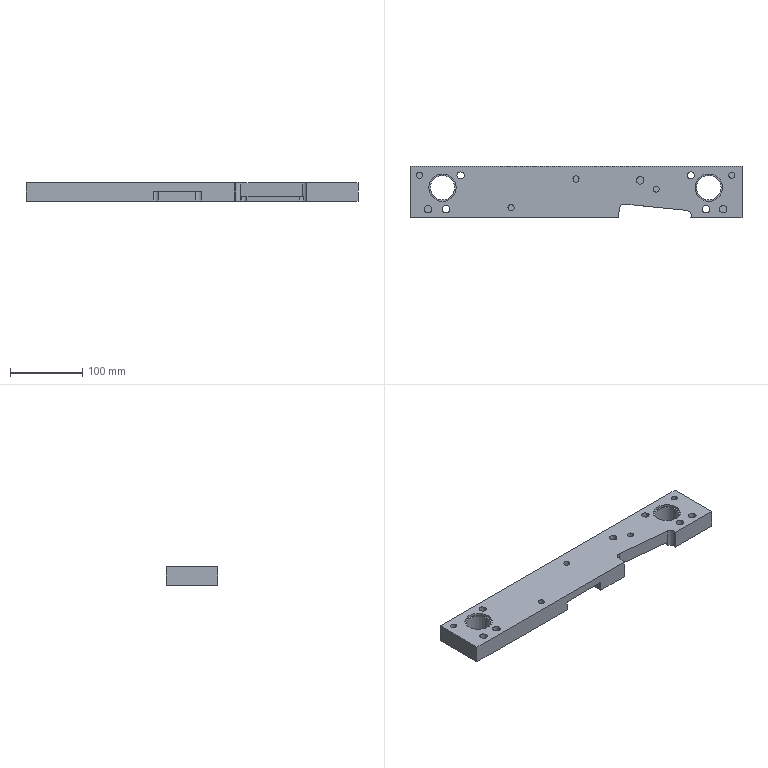Part | NX | features LIN_SOLID_COLOR 2 | 1 solid | 54 faces | box 460 x 72 x 25 mm | volume 694887 mm3 | plane 30 | cylinder 24 | commonest cylinder face diameters 8.5 x5 10.3 x5 10 x4 10.001 x2 10.31 x2 14 x2
STEP:
#1=CARTESIAN_POINT('',(698.25,138.,7.));
#2=VERTEX_POINT('',#1);
#3=CARTESIAN_POINT('',(694.,138.,7.));
#4=DIRECTION('',(0.,0.,1.));
#5=DIRECTION('',(1.,0.,0.));
#6=AXIS2_PLACEMENT_3D('',#3,#4,#5);
#7=CIRCLE('',#6,4.25);
#8=EDGE_CURVE('',#2,#2,#7,.F.);
#9=ORIENTED_EDGE('',*,*,#8,.T.);
#10=EDGE_LOOP('',(#9));
#11=FACE_BOUND('',#10,.T.);
#12=CARTESIAN_POINT('',(698.25,138.,25.));
#13=VERTEX_POINT('',#12);
#14=CARTESIAN_POINT('',(694.,138.,25.));
#15=DIRECTION('',(0.,0.,1.));
#16=DIRECTION('',(1.,0.,0.));
#17=AXIS2_PLACEMENT_3D('',#14,#15,#16);
#18=CIRCLE('',#17,4.25);
#19=EDGE_CURVE('',#13,#13,#18,.T.);
#20=ORIENTED_EDGE('',*,*,#19,.T.);
#21=EDGE_LOOP('',(#20));
#22=FACE_BOUND('',#21,.T.);
#23=CARTESIAN_POINT('',(694.,138.,25.1));
#24=DIRECTION('',(0.,0.,-1.));
#25=DIRECTION('',(1.,0.,0.));
#26=AXIS2_PLACEMENT_3D('',#23,#24,#25);
#27=CYLINDRICAL_SURFACE('',#26,4.25);
#28=ADVANCED_FACE('',(#11,#22),#27,.F.);
#29=CARTESIAN_POINT('',(747.152,157.,0.));
#30=VERTEX_POINT('',#29);
#31=CARTESIAN_POINT('',(741.997,157.,0.));
#32=DIRECTION('',(0.,0.,1.));
#33=DIRECTION('',(1.,0.,0.));
#34=AXIS2_PLACEMENT_3D('',#31,#32,#33);
#35=CIRCLE('',#34,5.155);
#36=EDGE_CURVE('',#30,#30,#35,.T.);
#37=ORIENTED_EDGE('',*,*,#36,.T.);
#38=EDGE_LOOP('',(#37));
#39=FACE_BOUND('',#38,.T.);
#40=CARTESIAN_POINT('',(428.158,157.,0.));
#41=VERTEX_POINT('',#40);
#42=CARTESIAN_POINT('',(423.003,157.,0.));
#43=DIRECTION('',(0.,0.,1.));
#44=DIRECTION('',(1.,0.,0.));
#45=AXIS2_PLACEMENT_3D('',#42,#43,#44);
#46=CIRCLE('',#45,5.155);
#47=EDGE_CURVE('',#41,#41,#46,.T.);
#48=ORIENTED_EDGE('',*,*,#47,.T.);
#49=EDGE_LOOP('',(#48));
#50=FACE_BOUND('',#49,.T.);
#51=CARTESIAN_POINT('',(757.85,110.,0.));
#52=VERTEX_POINT('',#51);
#53=CARTESIAN_POINT('',(763.,110.,0.));
#54=DIRECTION('',(0.,0.,-1.));
#55=DIRECTION('',(-1.,0.,0.));
#56=AXIS2_PLACEMENT_3D('',#53,#54,#55);
#57=CIRCLE('',#56,5.15);
#58=EDGE_CURVE('',#52,#52,#57,.T.);
#59=ORIENTED_EDGE('',*,*,#58,.F.);
#60=EDGE_LOOP('',(#59));
#61=FACE_BOUND('',#60,.T.);
#62=CARTESIAN_POINT('',(397.85,110.,0.));
#63=VERTEX_POINT('',#62);
#64=CARTESIAN_POINT('',(403.,110.,0.));
#65=DIRECTION('',(0.,0.,-1.));
#66=DIRECTION('',(-1.,0.,0.));
#67=AXIS2_PLACEMENT_3D('',#64,#65,#66);
#68=CIRCLE('',#67,5.15);
#69=EDGE_CURVE('',#63,#63,#68,.T.);
#70=ORIENTED_EDGE('',*,*,#69,.F.);
#71=EDGE_LOOP('',(#70));
#72=FACE_BOUND('',#71,.T.);
#73=CARTESIAN_POINT('',(381.,140.,0.));
#74=VERTEX_POINT('',#73);
#75=CARTESIAN_POINT('',(398.,140.,0.));
#76=DIRECTION('',(0.,0.,-1.));
#77=DIRECTION('',(-1.,0.,0.));
#78=AXIS2_PLACEMENT_3D('',#75,#76,#77);
#79=CIRCLE('',#78,17.);
#80=EDGE_CURVE('',#74,#74,#79,.T.);
#81=ORIENTED_EDGE('',*,*,#80,.F.);
#82=EDGE_LOOP('',(#81));
#83=FACE_BOUND('',#82,.T.);
#84=CARTESIAN_POINT('',(750.,140.,0.));
#85=VERTEX_POINT('',#84);
#86=CARTESIAN_POINT('',(767.,140.,0.));
#87=DIRECTION('',(0.,0.,-1.));
#88=DIRECTION('',(-1.,0.,0.));
#89=AXIS2_PLACEMENT_3D('',#86,#87,#88);
#90=CIRCLE('',#89,17.);
#91=EDGE_CURVE('',#85,#85,#90,.T.);
#92=ORIENTED_EDGE('',*,*,#91,.F.);
#93=EDGE_LOOP('',(#92));
#94=FACE_BOUND('',#93,.T.);
#95=CARTESIAN_POINT('',(650.988,129.15,0.));
#96=VERTEX_POINT('',#95);
#97=CARTESIAN_POINT('',(658.697,135.448,0.));
#98=VERTEX_POINT('',#97);
#99=CARTESIAN_POINT('',(654.541,132.668,0.));
#100=DIRECTION('',(0.,0.,-1.));
#101=DIRECTION('',(-1.,0.,0.));
#102=AXIS2_PLACEMENT_3D('',#99,#100,#101);
#103=CIRCLE('',#102,5.);
#104=EDGE_CURVE('',#96,#98,#103,.T.);
#105=ORIENTED_EDGE('',*,*,#104,.F.);
#106=CARTESIAN_POINT('',(649.783,117.177,0.));
#107=VERTEX_POINT('',#106);
#108=CARTESIAN_POINT('',(639.027,10.37,0.));
#109=DIRECTION('',(0.1002,0.995,0.));
#110=VECTOR('',#109,1000.);
#111=LINE('',#108,#110);
#112=EDGE_CURVE('',#107,#96,#111,.T.);
#113=ORIENTED_EDGE('',*,*,#112,.F.);
#114=CARTESIAN_POINT('',(643.119,110.885,0.));
#115=VERTEX_POINT('',#114);
#116=CARTESIAN_POINT('',(650.083,110.184,0.));
#117=DIRECTION('',(0.,0.,-1.));
#118=DIRECTION('',(-1.,0.,0.));
#119=AXIS2_PLACEMENT_3D('',#116,#117,#118);
#120=CIRCLE('',#119,7.);
#121=EDGE_CURVE('',#115,#107,#120,.T.);
#122=ORIENTED_EDGE('',*,*,#121,.F.);
#123=CARTESIAN_POINT('',(641.821,98.,0.));
#124=VERTEX_POINT('',#123);
#125=CARTESIAN_POINT('',(633.057,10.971,0.));
#126=DIRECTION('',(0.1002,0.995,0.));
#127=VECTOR('',#126,1000.);
#128=LINE('',#125,#127);
#129=EDGE_CURVE('',#124,#115,#128,.T.);
#130=ORIENTED_EDGE('',*,*,#129,.F.);
#131=CARTESIAN_POINT('',(595.5,98.,0.));
#132=VERTEX_POINT('',#131);
#133=CARTESIAN_POINT('',(742.,98.,0.));
#134=DIRECTION('',(-1.,0.,0.));
#135=VECTOR('',#134,1000.);
#136=LINE('',#133,#135);
#137=EDGE_CURVE('',#124,#132,#136,.T.);
#138=ORIENTED_EDGE('',*,*,#137,.T.);
#139=CARTESIAN_POINT('',(595.5,111.161,0.));
#140=VERTEX_POINT('',#139);
#141=CARTESIAN_POINT('',(595.5,0.,0.));
#142=DIRECTION('',(0.,1.,0.));
#143=VECTOR('',#142,1000.);
#144=LINE('',#141,#143);
#145=EDGE_CURVE('',#132,#140,#144,.T.);
#146=ORIENTED_EDGE('',*,*,#145,.T.);
#147=CARTESIAN_POINT('',(588.461,118.2,0.));
#148=VERTEX_POINT('',#147);
#149=CARTESIAN_POINT('',(592.318,115.018,0.));
#150=DIRECTION('',(0.,0.,-1.));
#151=DIRECTION('',(-1.,0.,0.));
#152=AXIS2_PLACEMENT_3D('',#149,#150,#151);
#153=CIRCLE('',#152,5.);
#154=EDGE_CURVE('',#140,#148,#153,.F.);
#155=ORIENTED_EDGE('',*,*,#154,.T.);
#156=CARTESIAN_POINT('',(536.539,118.2,0.));
#157=VERTEX_POINT('',#156);
#158=CARTESIAN_POINT('',(742.,118.2,0.));
#159=DIRECTION('',(-1.,0.,0.));
#160=VECTOR('',#159,1000.);
#161=LINE('',#158,#160);
#162=EDGE_CURVE('',#148,#157,#161,.T.);
#163=ORIENTED_EDGE('',*,*,#162,.T.);
#164=CARTESIAN_POINT('',(529.5,111.161,0.));
#165=VERTEX_POINT('',#164);
#166=CARTESIAN_POINT('',(532.682,115.018,0.));
#167=DIRECTION('',(0.,0.,-1.));
#168=DIRECTION('',(-1.,0.,0.));
#169=AXIS2_PLACEMENT_3D('',#166,#167,#168);
#170=CIRCLE('',#169,5.);
#171=EDGE_CURVE('',#157,#165,#170,.F.);
#172=ORIENTED_EDGE('',*,*,#171,.T.);
#173=CARTESIAN_POINT('',(529.5,98.,0.));
#174=VERTEX_POINT('',#173);
#175=CARTESIAN_POINT('',(529.5,0.,0.));
#176=DIRECTION('',(0.,-1.,0.));
#177=VECTOR('',#176,1000.);
#178=LINE('',#175,#177);
#179=EDGE_CURVE('',#165,#174,#178,.T.);
#180=ORIENTED_EDGE('',*,*,#179,.T.);
#181=CARTESIAN_POINT('',(353.,98.,0.));
#182=VERTEX_POINT('',#181);
#183=CARTESIAN_POINT('',(742.,98.,0.));
#184=DIRECTION('',(-1.,0.,0.));
#185=VECTOR('',#184,1000.);
#186=LINE('',#183,#185);
#187=EDGE_CURVE('',#174,#182,#186,.T.);
#188=ORIENTED_EDGE('',*,*,#187,.T.);
#189=CARTESIAN_POINT('',(353.,170.,0.));
#190=VERTEX_POINT('',#189);
#191=CARTESIAN_POINT('',(353.,0.,0.));
#192=DIRECTION('',(0.,-1.,0.));
#193=VECTOR('',#192,1000.);
#194=LINE('',#191,#193);
#195=EDGE_CURVE('',#190,#182,#194,.T.);
#196=ORIENTED_EDGE('',*,*,#195,.F.);
#197=CARTESIAN_POINT('',(813.,170.,0.));
#198=VERTEX_POINT('',#197);
#199=CARTESIAN_POINT('',(788.,170.,0.));
#200=DIRECTION('',(-1.,0.,0.));
#201=VECTOR('',#200,1000.);
#202=LINE('',#199,#201);
#203=EDGE_CURVE('',#198,#190,#202,.T.);
#204=ORIENTED_EDGE('',*,*,#203,.F.);
#205=CARTESIAN_POINT('',(813.,98.,0.));
#206=VERTEX_POINT('',#205);
#207=CARTESIAN_POINT('',(813.,0.,0.));
#208=DIRECTION('',(0.,-1.,0.));
#209=VECTOR('',#208,1000.);
#210=LINE('',#207,#209);
#211=EDGE_CURVE('',#198,#206,#210,.T.);
#212=ORIENTED_EDGE('',*,*,#211,.T.);
#213=CARTESIAN_POINT('',(742.327,98.,0.));
#214=VERTEX_POINT('',#213);
#215=CARTESIAN_POINT('',(742.,98.,0.));
#216=DIRECTION('',(-1.,0.,0.));
#217=VECTOR('',#216,1000.);
#218=LINE('',#215,#217);
#219=EDGE_CURVE('',#206,#214,#218,.T.);
#220=ORIENTED_EDGE('',*,*,#219,.T.);
#221=CARTESIAN_POINT('',(742.615,100.865,0.));
#222=VERTEX_POINT('',#221);
#223=CARTESIAN_POINT('',(732.553,0.9513,0.));
#224=DIRECTION('',(-0.1002,-0.995,0.));
#225=VECTOR('',#224,1000.);
#226=LINE('',#223,#225);
#227=EDGE_CURVE('',#222,#214,#226,.T.);
#228=ORIENTED_EDGE('',*,*,#227,.F.);
#229=CARTESIAN_POINT('',(737.34,108.36,0.));
#230=VERTEX_POINT('',#229);
#231=CARTESIAN_POINT('',(735.651,101.567,0.));
#232=DIRECTION('',(0.,0.,-1.));
#233=DIRECTION('',(-1.,0.,0.));
#234=AXIS2_PLACEMENT_3D('',#231,#232,#233);
#235=CIRCLE('',#234,7.);
#236=EDGE_CURVE('',#230,#222,#235,.T.);
#237=ORIENTED_EDGE('',*,*,#236,.F.);
#238=CARTESIAN_POINT('',(738.545,120.332,0.));
#239=VERTEX_POINT('',#238);
#240=CARTESIAN_POINT('',(726.584,1.552,0.));
#241=DIRECTION('',(-0.1002,-0.995,0.));
#242=VECTOR('',#241,1000.);
#243=LINE('',#240,#242);
#244=EDGE_CURVE('',#239,#230,#243,.T.);
#245=ORIENTED_EDGE('',*,*,#244,.F.);
#246=CARTESIAN_POINT('',(732.247,128.041,0.));
#247=VERTEX_POINT('',#246);
#248=CARTESIAN_POINT('',(735.766,124.489,0.));
#249=DIRECTION('',(0.,0.,-1.));
#250=DIRECTION('',(-1.,0.,0.));
#251=AXIS2_PLACEMENT_3D('',#248,#249,#250);
#252=CIRCLE('',#251,5.);
#253=EDGE_CURVE('',#247,#239,#252,.T.);
#254=ORIENTED_EDGE('',*,*,#253,.F.);
#255=CARTESIAN_POINT('',(754.667,125.783,0.));
#256=DIRECTION('',(0.995,-0.1002,0.));
#257=VECTOR('',#256,1000.);
#258=LINE('',#255,#257);
#259=EDGE_CURVE('',#98,#247,#258,.T.);
#260=ORIENTED_EDGE('',*,*,#259,.F.);
#261=EDGE_LOOP('',(#105,#113,#122,#130,#138,#146,#155,#163,#172,#180,#188,#196,#204,#212,#220,#228,#237,#245,#254,#260));
#262=FACE_BOUND('',#261,.T.);
#263=CARTESIAN_POINT('',(742.,0.,0.));
#264=DIRECTION('',(0.,0.,-1.));
#265=DIRECTION('',(-1.,0.,0.));
#266=AXIS2_PLACEMENT_3D('',#263,#264,#265);
#267=PLANE('',#266);
#268=ADVANCED_FACE('',(#39,#50,#61,#72,#83,#94,#262),#267,.T.);
#269=CARTESIAN_POINT('',(587.25,152.,1.));
#270=VERTEX_POINT('',#269);
#271=CARTESIAN_POINT('',(583.,152.,1.));
#272=DIRECTION('',(0.,0.,1.));
#273=DIRECTION('',(1.,0.,0.));
#274=AXIS2_PLACEMENT_3D('',#271,#272,#273);
#275=CIRCLE('',#274,4.25);
#276=EDGE_CURVE('',#270,#270,#275,.F.);
#277=ORIENTED_EDGE('',*,*,#276,.T.);
#278=EDGE_LOOP('',(#277));
#279=FACE_BOUND('',#278,.T.);
#280=CARTESIAN_POINT('',(587.25,152.,25.));
#281=VERTEX_POINT('',#280);
#282=CARTESIAN_POINT('',(583.,152.,25.));
#283=DIRECTION('',(0.,0.,1.));
#284=DIRECTION('',(1.,0.,0.));
#285=AXIS2_PLACEMENT_3D('',#282,#283,#284);
#286=CIRCLE('',#285,4.25);
#287=EDGE_CURVE('',#281,#281,#286,.T.);
#288=ORIENTED_EDGE('',*,*,#287,.T.);
#289=EDGE_LOOP('',(#288));
#290=FACE_BOUND('',#289,.T.);
#291=CARTESIAN_POINT('',(583.,152.,25.1));
#292=DIRECTION('',(0.,0.,-1.));
#293=DIRECTION('',(1.,0.,0.));
#294=AXIS2_PLACEMENT_3D('',#291,#292,#293);
#295=CYLINDRICAL_SURFACE('',#294,4.25);
#296=ADVANCED_FACE('',(#279,#290),#295,.F.);
#297=CARTESIAN_POINT('',(595.5,111.161,13.5));
#298=VERTEX_POINT('',#297);
#299=CARTESIAN_POINT('',(588.461,118.2,13.5));
#300=VERTEX_POINT('',#299);
#301=CARTESIAN_POINT('',(592.318,115.018,13.5));
#302=DIRECTION('',(0.,0.,1.));
#303=DIRECTION('',(1.,0.,0.));
#304=AXIS2_PLACEMENT_3D('',#301,#302,#303);
#305=CIRCLE('',#304,5.);
#306=EDGE_CURVE('',#298,#300,#305,.T.);
#307=ORIENTED_EDGE('',*,*,#306,.F.);
#308=CARTESIAN_POINT('',(595.5,98.,13.5));
#309=VERTEX_POINT('',#308);
#310=CARTESIAN_POINT('',(595.5,90.2,13.5));
#311=DIRECTION('',(0.,1.,0.));
#312=VECTOR('',#311,1000.);
#313=LINE('',#310,#312);
#314=EDGE_CURVE('',#309,#298,#313,.T.);
#315=ORIENTED_EDGE('',*,*,#314,.F.);
#316=CARTESIAN_POINT('',(529.5,98.,13.5));
#317=VERTEX_POINT('',#316);
#318=CARTESIAN_POINT('',(915.758,98.,13.5));
#319=DIRECTION('',(-1.,0.,0.));
#320=VECTOR('',#319,1000.);
#321=LINE('',#318,#320);
#322=EDGE_CURVE('',#309,#317,#321,.T.);
#323=ORIENTED_EDGE('',*,*,#322,.T.);
#324=CARTESIAN_POINT('',(529.5,111.161,13.5));
#325=VERTEX_POINT('',#324);
#326=CARTESIAN_POINT('',(529.5,110.2,13.5));
#327=DIRECTION('',(0.,-1.,0.));
#328=VECTOR('',#327,1000.);
#329=LINE('',#326,#328);
#330=EDGE_CURVE('',#325,#317,#329,.T.);
#331=ORIENTED_EDGE('',*,*,#330,.F.);
#332=CARTESIAN_POINT('',(536.539,118.2,13.5));
#333=VERTEX_POINT('',#332);
#334=CARTESIAN_POINT('',(532.682,115.018,13.5));
#335=DIRECTION('',(0.,0.,1.));
#336=DIRECTION('',(1.,0.,0.));
#337=AXIS2_PLACEMENT_3D('',#334,#335,#336);
#338=CIRCLE('',#337,5.);
#339=EDGE_CURVE('',#333,#325,#338,.T.);
#340=ORIENTED_EDGE('',*,*,#339,.F.);
#341=CARTESIAN_POINT('',(572.,118.2,13.5));
#342=DIRECTION('',(-1.,0.,0.));
#343=VECTOR('',#342,1000.);
#344=LINE('',#341,#343);
#345=EDGE_CURVE('',#300,#333,#344,.T.);
#346=ORIENTED_EDGE('',*,*,#345,.F.);
#347=EDGE_LOOP('',(#307,#315,#323,#331,#340,#346));
#348=FACE_BOUND('',#347,.T.);
#349=CARTESIAN_POINT('',(552.555,107.951,13.5));
#350=DIRECTION('',(0.,0.,1.));
#351=DIRECTION('',(1.,0.,0.));
#352=AXIS2_PLACEMENT_3D('',#349,#350,#351);
#353=PLANE('',#352);
#354=ADVANCED_FACE('',(#348),#353,.F.);
#355=CARTESIAN_POINT('',(415.,140.,21.7));
#356=VERTEX_POINT('',#355);
#357=CARTESIAN_POINT('',(398.,140.,21.7));
#358=DIRECTION('',(0.,0.,1.));
#359=DIRECTION('',(1.,0.,0.));
#360=AXIS2_PLACEMENT_3D('',#357,#358,#359);
#361=CIRCLE('',#360,17.);
#362=EDGE_CURVE('',#356,#356,#361,.F.);
#363=ORIENTED_EDGE('',*,*,#362,.T.);
#364=EDGE_LOOP('',(#363));
#365=FACE_BOUND('',#364,.T.);
#366=CARTESIAN_POINT('',(417.,140.,21.7));
#367=VERTEX_POINT('',#366);
#368=CARTESIAN_POINT('',(398.,140.,21.7));
#369=DIRECTION('',(0.,0.,1.));
#370=DIRECTION('',(1.,0.,0.));
#371=AXIS2_PLACEMENT_3D('',#368,#369,#370);
#372=CIRCLE('',#371,19.);
#373=EDGE_CURVE('',#367,#367,#372,.F.);
#374=ORIENTED_EDGE('',*,*,#373,.F.);
#375=EDGE_LOOP('',(#374));
#376=FACE_BOUND('',#375,.T.);
#377=CARTESIAN_POINT('',(398.,140.,21.7));
#378=DIRECTION('',(0.,0.,1.));
#379=DIRECTION('',(1.,0.,0.));
#380=AXIS2_PLACEMENT_3D('',#377,#378,#379);
#381=PLANE('',#380);
#382=ADVANCED_FACE('',(#365,#376),#381,.T.);
#383=CARTESIAN_POINT('',(784.,140.,21.7));
#384=VERTEX_POINT('',#383);
#385=CARTESIAN_POINT('',(767.,140.,21.7));
#386=DIRECTION('',(0.,0.,1.));
#387=DIRECTION('',(1.,0.,0.));
#388=AXIS2_PLACEMENT_3D('',#385,#386,#387);
#389=CIRCLE('',#388,17.);
#390=EDGE_CURVE('',#384,#384,#389,.F.);
#391=ORIENTED_EDGE('',*,*,#390,.T.);
#392=EDGE_LOOP('',(#391));
#393=FACE_BOUND('',#392,.T.);
#394=CARTESIAN_POINT('',(786.,140.,21.7));
#395=VERTEX_POINT('',#394);
#396=CARTESIAN_POINT('',(767.,140.,21.7));
#397=DIRECTION('',(0.,0.,1.));
#398=DIRECTION('',(1.,0.,0.));
#399=AXIS2_PLACEMENT_3D('',#396,#397,#398);
#400=CIRCLE('',#399,19.);
#401=EDGE_CURVE('',#395,#395,#400,.F.);
#402=ORIENTED_EDGE('',*,*,#401,.F.);
#403=EDGE_LOOP('',(#402));
#404=FACE_BOUND('',#403,.T.);
#405=CARTESIAN_POINT('',(767.,140.,21.7));
#406=DIRECTION('',(0.,0.,1.));
#407=DIRECTION('',(1.,0.,0.));
#408=AXIS2_PLACEMENT_3D('',#405,#406,#407);
#409=PLANE('',#408);
#410=ADVANCED_FACE('',(#393,#404),#409,.T.);
#411=CARTESIAN_POINT('',(786.,140.,25.));
#412=VERTEX_POINT('',#411);
#413=CARTESIAN_POINT('',(767.,140.,25.));
#414=DIRECTION('',(0.,0.,1.));
#415=DIRECTION('',(1.,0.,0.));
#416=AXIS2_PLACEMENT_3D('',#413,#414,#415);
#417=CIRCLE('',#416,19.);
#418=EDGE_CURVE('',#412,#412,#417,.T.);
#419=ORIENTED_EDGE('',*,*,#418,.T.);
#420=EDGE_LOOP('',(#419));
#421=FACE_BOUND('',#420,.T.);
#422=ORIENTED_EDGE('',*,*,#401,.T.);
#423=EDGE_LOOP('',(#422));
#424=FACE_BOUND('',#423,.T.);
#425=CARTESIAN_POINT('',(767.,140.,21.5));
#426=DIRECTION('',(0.,0.,1.));
#427=DIRECTION('',(1.,0.,0.));
#428=AXIS2_PLACEMENT_3D('',#425,#426,#427);
#429=CYLINDRICAL_SURFACE('',#428,19.);
#430=ADVANCED_FACE('',(#421,#424),#429,.F.);
#431=CARTESIAN_POINT('',(417.,140.,25.));
#432=VERTEX_POINT('',#431);
#433=CARTESIAN_POINT('',(398.,140.,25.));
#434=DIRECTION('',(0.,0.,1.));
#435=DIRECTION('',(1.,0.,0.));
#436=AXIS2_PLACEMENT_3D('',#433,#434,#435);
#437=CIRCLE('',#436,19.);
#438=EDGE_CURVE('',#432,#432,#437,.T.);
#439=ORIENTED_EDGE('',*,*,#438,.T.);
#440=EDGE_LOOP('',(#439));
#441=FACE_BOUND('',#440,.T.);
#442=ORIENTED_EDGE('',*,*,#373,.T.);
#443=EDGE_LOOP('',(#442));
#444=FACE_BOUND('',#443,.T.);
#445=CARTESIAN_POINT('',(398.,140.,21.5));
#446=DIRECTION('',(0.,0.,1.));
#447=DIRECTION('',(1.,0.,0.));
#448=AXIS2_PLACEMENT_3D('',#445,#446,#447);
#449=CYLINDRICAL_SURFACE('',#448,19.);
#450=ADVANCED_FACE('',(#441,#444),#449,.F.);
#451=CARTESIAN_POINT('',(588.461,118.2,-46.5));
#452=DIRECTION('',(0.,0.,1.));
#453=VECTOR('',#452,1000.);
#454=LINE('',#451,#453);
#455=EDGE_CURVE('',#148,#300,#454,.T.);
#456=ORIENTED_EDGE('',*,*,#455,.T.);
#457=ORIENTED_EDGE('',*,*,#345,.T.);
#458=CARTESIAN_POINT('',(536.539,118.2,-46.5));
#459=DIRECTION('',(0.,0.,1.));
#460=VECTOR('',#459,1000.);
#461=LINE('',#458,#460);
#462=EDGE_CURVE('',#157,#333,#461,.T.);
#463=ORIENTED_EDGE('',*,*,#462,.F.);
#464=ORIENTED_EDGE('',*,*,#162,.F.);
#465=EDGE_LOOP('',(#456,#457,#463,#464));
#466=FACE_BOUND('',#465,.T.);
#467=CARTESIAN_POINT('',(572.,118.2,-46.5));
#468=DIRECTION('',(0.,-1.,0.));
#469=DIRECTION('',(0.,0.,1.));
#470=AXIS2_PLACEMENT_3D('',#467,#468,#469);
#471=PLANE('',#470);
#472=ADVANCED_FACE('',(#466),#471,.T.);
#473=CARTESIAN_POINT('',(595.5,111.161,-46.5));
#474=DIRECTION('',(0.,0.,1.));
#475=VECTOR('',#474,1000.);
#476=LINE('',#473,#475);
#477=EDGE_CURVE('',#140,#298,#476,.T.);
#478=ORIENTED_EDGE('',*,*,#477,.T.);
#479=ORIENTED_EDGE('',*,*,#306,.T.);
#480=ORIENTED_EDGE('',*,*,#455,.F.);
#481=ORIENTED_EDGE('',*,*,#154,.F.);
#482=EDGE_LOOP('',(#478,#479,#480,#481));
#483=FACE_BOUND('',#482,.T.);
#484=CARTESIAN_POINT('',(592.318,115.018,-46.5));
#485=DIRECTION('',(0.,0.,1.));
#486=DIRECTION('',(1.,0.,0.));
#487=AXIS2_PLACEMENT_3D('',#484,#485,#486);
#488=CYLINDRICAL_SURFACE('',#487,5.);
#489=ADVANCED_FACE('',(#483),#488,.F.);
#490=CARTESIAN_POINT('',(595.5,98.,0.));
#491=DIRECTION('',(0.,0.,-1.));
#492=VECTOR('',#491,1000.);
#493=LINE('',#490,#492);
#494=EDGE_CURVE('',#309,#132,#493,.T.);
#495=ORIENTED_EDGE('',*,*,#494,.F.);
#496=ORIENTED_EDGE('',*,*,#314,.T.);
#497=ORIENTED_EDGE('',*,*,#477,.F.);
#498=ORIENTED_EDGE('',*,*,#145,.F.);
#499=EDGE_LOOP('',(#495,#496,#497,#498));
#500=FACE_BOUND('',#499,.T.);
#501=CARTESIAN_POINT('',(595.5,90.2,-46.5));
#502=DIRECTION('',(-1.,0.,0.));
#503=DIRECTION('',(0.,0.,1.));
#504=AXIS2_PLACEMENT_3D('',#501,#502,#503);
#505=PLANE('',#504);
#506=ADVANCED_FACE('',(#500),#505,.T.);
#507=CARTESIAN_POINT('',(643.119,110.885,25.));
#508=VERTEX_POINT('',#507);
#509=CARTESIAN_POINT('',(641.821,98.,25.));
#510=VERTEX_POINT('',#509);
#511=CARTESIAN_POINT('',(633.519,15.557,25.));
#512=DIRECTION('',(-0.1002,-0.995,0.));
#513=VECTOR('',#512,1000.);
#514=LINE('',#511,#513);
#515=EDGE_CURVE('',#508,#510,#514,.T.);
#516=ORIENTED_EDGE('',*,*,#515,.T.);
#517=CARTESIAN_POINT('',(641.821,98.,0.));
#518=DIRECTION('',(0.,0.,-1.));
#519=VECTOR('',#518,1000.);
#520=LINE('',#517,#519);
#521=EDGE_CURVE('',#510,#124,#520,.T.);
#522=ORIENTED_EDGE('',*,*,#521,.T.);
#523=ORIENTED_EDGE('',*,*,#129,.T.);
#524=CARTESIAN_POINT('',(643.119,110.885,-41.49));
#525=DIRECTION('',(0.,0.,1.));
#526=VECTOR('',#525,1000.);
#527=LINE('',#524,#526);
#528=EDGE_CURVE('',#115,#508,#527,.T.);
#529=ORIENTED_EDGE('',*,*,#528,.T.);
#530=EDGE_LOOP('',(#516,#522,#523,#529));
#531=FACE_BOUND('',#530,.T.);
#532=CARTESIAN_POINT('',(643.119,110.885,-41.49));
#533=DIRECTION('',(-0.995,0.1002,0.));
#534=DIRECTION('',(-0.1002,-0.995,0.));
#535=AXIS2_PLACEMENT_3D('',#532,#533,#534);
#536=PLANE('',#535);
#537=ADVANCED_FACE('',(#531),#536,.F.);
#538=CARTESIAN_POINT('',(649.783,117.177,6.));
#539=VERTEX_POINT('',#538);
#540=CARTESIAN_POINT('',(649.783,117.177,-41.49));
#541=DIRECTION('',(0.,0.,1.));
#542=VECTOR('',#541,1000.);
#543=LINE('',#540,#542);
#544=EDGE_CURVE('',#107,#539,#543,.T.);
#545=ORIENTED_EDGE('',*,*,#544,.T.);
#546=CARTESIAN_POINT('',(650.785,117.149,6.));
#547=VERTEX_POINT('',#546);
#548=CARTESIAN_POINT('',(650.083,110.184,6.));
#549=DIRECTION('',(0.,0.,1.));
#550=DIRECTION('',(1.,0.,0.));
#551=AXIS2_PLACEMENT_3D('',#548,#549,#550);
#552=CIRCLE('',#551,7.);
#553=EDGE_CURVE('',#539,#547,#552,.F.);
#554=ORIENTED_EDGE('',*,*,#553,.T.);
#555=CARTESIAN_POINT('',(650.785,117.149,25.));
#556=VERTEX_POINT('',#555);
#557=CARTESIAN_POINT('',(650.785,117.149,-41.49));
#558=DIRECTION('',(0.,0.,1.));
#559=VECTOR('',#558,1000.);
#560=LINE('',#557,#559);
#561=EDGE_CURVE('',#556,#547,#560,.F.);
#562=ORIENTED_EDGE('',*,*,#561,.F.);
#563=CARTESIAN_POINT('',(650.083,110.184,25.));
#564=DIRECTION('',(0.,0.,1.));
#565=DIRECTION('',(1.,0.,0.));
#566=AXIS2_PLACEMENT_3D('',#563,#564,#565);
#567=CIRCLE('',#566,7.);
#568=EDGE_CURVE('',#556,#508,#567,.T.);
#569=ORIENTED_EDGE('',*,*,#568,.T.);
#570=ORIENTED_EDGE('',*,*,#528,.F.);
#571=ORIENTED_EDGE('',*,*,#121,.T.);
#572=EDGE_LOOP('',(#545,#554,#562,#569,#570,#571));
#573=FACE_BOUND('',#572,.T.);
#574=CARTESIAN_POINT('',(650.083,110.184,-41.49));
#575=DIRECTION('',(0.,0.,1.));
#576=DIRECTION('',(1.,0.,0.));
#577=AXIS2_PLACEMENT_3D('',#574,#575,#576);
#578=CYLINDRICAL_SURFACE('',#577,7.);
#579=ADVANCED_FACE('',(#573),#578,.F.);
#580=CARTESIAN_POINT('',(736.352,108.532,6.));
#581=VERTEX_POINT('',#580);
#582=CARTESIAN_POINT('',(652.775,116.948,6.));
#583=DIRECTION('',(-0.995,0.1002,0.));
#584=VECTOR('',#583,1000.);
#585=LINE('',#582,#584);
#586=EDGE_CURVE('',#581,#547,#585,.T.);
#587=ORIENTED_EDGE('',*,*,#586,.F.);
#588=CARTESIAN_POINT('',(736.352,108.532,25.));
#589=VERTEX_POINT('',#588);
#590=CARTESIAN_POINT('',(736.352,108.532,-41.49));
#591=DIRECTION('',(0.,0.,1.));
#592=VECTOR('',#591,1000.);
#593=LINE('',#590,#592);
#594=EDGE_CURVE('',#581,#589,#593,.T.);
#595=ORIENTED_EDGE('',*,*,#594,.T.);
#596=CARTESIAN_POINT('',(798.301,102.293,25.));
#597=DIRECTION('',(0.995,-0.1002,0.));
#598=VECTOR('',#597,1000.);
#599=LINE('',#596,#598);
#600=EDGE_CURVE('',#556,#589,#599,.T.);
#601=ORIENTED_EDGE('',*,*,#600,.F.);
#602=ORIENTED_EDGE('',*,*,#561,.T.);
#603=EDGE_LOOP('',(#587,#595,#601,#602));
#604=FACE_BOUND('',#603,.T.);
#605=CARTESIAN_POINT('',(652.775,116.948,-41.49));
#606=DIRECTION('',(-0.1002,-0.995,0.));
#607=DIRECTION('',(0.995,-0.1002,0.));
#608=AXIS2_PLACEMENT_3D('',#605,#606,#607);
#609=PLANE('',#608);
#610=ADVANCED_FACE('',(#604),#609,.T.);
#611=ORIENTED_EDGE('',*,*,#594,.F.);
#612=CARTESIAN_POINT('',(737.34,108.36,6.));
#613=VERTEX_POINT('',#612);
#614=CARTESIAN_POINT('',(735.651,101.567,6.));
#615=DIRECTION('',(0.,0.,1.));
#616=DIRECTION('',(1.,0.,0.));
#617=AXIS2_PLACEMENT_3D('',#614,#615,#616);
#618=CIRCLE('',#617,7.);
#619=EDGE_CURVE('',#581,#613,#618,.F.);
#620=ORIENTED_EDGE('',*,*,#619,.T.);
#621=CARTESIAN_POINT('',(737.34,108.36,-41.49));
#622=DIRECTION('',(0.,0.,-1.));
#623=VECTOR('',#622,1000.);
#624=LINE('',#621,#623);
#625=EDGE_CURVE('',#613,#230,#624,.T.);
#626=ORIENTED_EDGE('',*,*,#625,.T.);
#627=ORIENTED_EDGE('',*,*,#236,.T.);
#628=CARTESIAN_POINT('',(742.615,100.865,25.));
#629=VERTEX_POINT('',#628);
#630=CARTESIAN_POINT('',(742.615,100.865,-41.49));
#631=DIRECTION('',(0.,0.,1.));
#632=VECTOR('',#631,1000.);
#633=LINE('',#630,#632);
#634=EDGE_CURVE('',#629,#222,#633,.F.);
#635=ORIENTED_EDGE('',*,*,#634,.F.);
#636=CARTESIAN_POINT('',(735.651,101.567,25.));
#637=DIRECTION('',(0.,0.,1.));
#638=DIRECTION('',(1.,0.,0.));
#639=AXIS2_PLACEMENT_3D('',#636,#637,#638);
#640=CIRCLE('',#639,7.);
#641=EDGE_CURVE('',#629,#589,#640,.T.);
#642=ORIENTED_EDGE('',*,*,#641,.T.);
#643=EDGE_LOOP('',(#611,#620,#626,#627,#635,#642));
#644=FACE_BOUND('',#643,.T.);
#645=CARTESIAN_POINT('',(735.651,101.567,-41.49));
#646=DIRECTION('',(0.,0.,-1.));
#647=DIRECTION('',(-1.,0.,0.));
#648=AXIS2_PLACEMENT_3D('',#645,#646,#647);
#649=CYLINDRICAL_SURFACE('',#648,7.);
#650=ADVANCED_FACE('',(#644),#649,.F.);
#651=CARTESIAN_POINT('',(742.327,98.,25.));
#652=VERTEX_POINT('',#651);
#653=CARTESIAN_POINT('',(733.015,5.537,25.));
#654=DIRECTION('',(0.1002,0.995,0.));
#655=VECTOR('',#654,1000.);
#656=LINE('',#653,#655);
#657=EDGE_CURVE('',#652,#629,#656,.T.);
#658=ORIENTED_EDGE('',*,*,#657,.T.);
#659=ORIENTED_EDGE('',*,*,#634,.T.);
#660=ORIENTED_EDGE('',*,*,#227,.T.);
#661=CARTESIAN_POINT('',(742.327,98.,0.));
#662=DIRECTION('',(0.,0.,1.));
#663=VECTOR('',#662,1000.);
#664=LINE('',#661,#663);
#665=EDGE_CURVE('',#214,#652,#664,.T.);
#666=ORIENTED_EDGE('',*,*,#665,.T.);
#667=EDGE_LOOP('',(#658,#659,#660,#666));
#668=FACE_BOUND('',#667,.T.);
#669=CARTESIAN_POINT('',(742.615,100.865,-41.49));
#670=DIRECTION('',(0.995,-0.1002,0.));
#671=DIRECTION('',(0.1002,0.995,0.));
#672=AXIS2_PLACEMENT_3D('',#669,#670,#671);
#673=PLANE('',#672);
#674=ADVANCED_FACE('',(#668),#673,.F.);
#675=ORIENTED_EDGE('',*,*,#665,.F.);
#676=ORIENTED_EDGE('',*,*,#219,.F.);
#677=CARTESIAN_POINT('',(813.,98.,25.));
#678=VERTEX_POINT('',#677);
#679=CARTESIAN_POINT('',(813.,98.,12.5));
#680=DIRECTION('',(0.,0.,-1.));
#681=VECTOR('',#680,1000.);
#682=LINE('',#679,#681);
#683=EDGE_CURVE('',#678,#206,#682,.T.);
#684=ORIENTED_EDGE('',*,*,#683,.F.);
#685=CARTESIAN_POINT('',(788.,98.,25.));
#686=DIRECTION('',(1.,0.,0.));
#687=VECTOR('',#686,1000.);
#688=LINE('',#685,#687);
#689=EDGE_CURVE('',#652,#678,#688,.T.);
#690=ORIENTED_EDGE('',*,*,#689,.F.);
#691=EDGE_LOOP('',(#675,#676,#684,#690));
#692=FACE_BOUND('',#691,.T.);
#693=CARTESIAN_POINT('',(915.758,98.,0.));
#694=DIRECTION('',(0.,-1.,0.));
#695=DIRECTION('',(0.,0.,-1.));
#696=AXIS2_PLACEMENT_3D('',#693,#694,#695);
#697=PLANE('',#696);
#698=ADVANCED_FACE('',(#692),#697,.T.);
#699=CARTESIAN_POINT('',(813.,170.,25.));
#700=VERTEX_POINT('',#699);
#701=CARTESIAN_POINT('',(813.,0.,25.));
#702=DIRECTION('',(0.,1.,0.));
#703=VECTOR('',#702,1000.);
#704=LINE('',#701,#703);
#705=EDGE_CURVE('',#678,#700,#704,.T.);
#706=ORIENTED_EDGE('',*,*,#705,.F.);
#707=ORIENTED_EDGE('',*,*,#683,.T.);
#708=ORIENTED_EDGE('',*,*,#211,.F.);
#709=CARTESIAN_POINT('',(813.,170.,25.));
#710=DIRECTION('',(0.,0.,-1.));
#711=VECTOR('',#710,1000.);
#712=LINE('',#709,#711);
#713=EDGE_CURVE('',#700,#198,#712,.T.);
#714=ORIENTED_EDGE('',*,*,#713,.F.);
#715=EDGE_LOOP('',(#706,#707,#708,#714));
#716=FACE_BOUND('',#715,.T.);
#717=CARTESIAN_POINT('',(813.,0.,12.5));
#718=DIRECTION('',(1.,0.,0.));
#719=DIRECTION('',(0.,0.,-1.));
#720=AXIS2_PLACEMENT_3D('',#717,#718,#719);
#721=PLANE('',#720);
#722=ADVANCED_FACE('',(#716),#721,.T.);
#723=CARTESIAN_POINT('',(353.,170.,25.));
#724=VERTEX_POINT('',#723);
#725=CARTESIAN_POINT('',(788.,170.,25.));
#726=DIRECTION('',(1.,0.,0.));
#727=VECTOR('',#726,1000.);
#728=LINE('',#725,#727);
#729=EDGE_CURVE('',#724,#700,#728,.T.);
#730=ORIENTED_EDGE('',*,*,#729,.T.);
#731=ORIENTED_EDGE('',*,*,#713,.T.);
#732=ORIENTED_EDGE('',*,*,#203,.T.);
#733=CARTESIAN_POINT('',(353.,170.,25.));
#734=DIRECTION('',(0.,0.,1.));
#735=VECTOR('',#734,1000.);
#736=LINE('',#733,#735);
#737=EDGE_CURVE('',#190,#724,#736,.T.);
#738=ORIENTED_EDGE('',*,*,#737,.T.);
#739=EDGE_LOOP('',(#730,#731,#732,#738));
#740=FACE_BOUND('',#739,.T.);
#741=CARTESIAN_POINT('',(788.,170.,25.));
#742=DIRECTION('',(0.,1.,0.));
#743=DIRECTION('',(0.,0.,1.));
#744=AXIS2_PLACEMENT_3D('',#741,#742,#743);
#745=PLANE('',#744);
#746=ADVANCED_FACE('',(#740),#745,.T.);
#747=ORIENTED_EDGE('',*,*,#195,.T.);
#748=CARTESIAN_POINT('',(353.,98.,25.));
#749=VERTEX_POINT('',#748);
#750=CARTESIAN_POINT('',(353.,98.,25.));
#751=DIRECTION('',(0.,0.,1.));
#752=VECTOR('',#751,1000.);
#753=LINE('',#750,#752);
#754=EDGE_CURVE('',#182,#749,#753,.T.);
#755=ORIENTED_EDGE('',*,*,#754,.T.);
#756=CARTESIAN_POINT('',(353.,0.,25.));
#757=DIRECTION('',(0.,1.,0.));
#758=VECTOR('',#757,1000.);
#759=LINE('',#756,#758);
#760=EDGE_CURVE('',#749,#724,#759,.T.);
#761=ORIENTED_EDGE('',*,*,#760,.T.);
#762=ORIENTED_EDGE('',*,*,#737,.F.);
#763=EDGE_LOOP('',(#747,#755,#761,#762));
#764=FACE_BOUND('',#763,.T.);
#765=CARTESIAN_POINT('',(353.,0.,25.));
#766=DIRECTION('',(-1.,0.,0.));
#767=DIRECTION('',(0.,0.,1.));
#768=AXIS2_PLACEMENT_3D('',#765,#766,#767);
#769=PLANE('',#768);
#770=ADVANCED_FACE('',(#764),#769,.T.);
#771=CARTESIAN_POINT('',(529.5,98.,-46.5));
#772=DIRECTION('',(0.,0.,-1.));
#773=VECTOR('',#772,1000.);
#774=LINE('',#771,#773);
#775=EDGE_CURVE('',#317,#174,#774,.T.);
#776=ORIENTED_EDGE('',*,*,#775,.F.);
#777=ORIENTED_EDGE('',*,*,#322,.F.);
#778=ORIENTED_EDGE('',*,*,#494,.T.);
#779=ORIENTED_EDGE('',*,*,#137,.F.);
#780=ORIENTED_EDGE('',*,*,#521,.F.);
#781=CARTESIAN_POINT('',(788.,98.,25.));
#782=DIRECTION('',(1.,0.,0.));
#783=VECTOR('',#782,1000.);
#784=LINE('',#781,#783);
#785=EDGE_CURVE('',#749,#510,#784,.T.);
#786=ORIENTED_EDGE('',*,*,#785,.F.);
#787=ORIENTED_EDGE('',*,*,#754,.F.);
#788=ORIENTED_EDGE('',*,*,#187,.F.);
#789=EDGE_LOOP('',(#776,#777,#778,#779,#780,#786,#787,#788));
#790=FACE_BOUND('',#789,.T.);
#791=CARTESIAN_POINT('',(915.758,98.,0.));
#792=DIRECTION('',(0.,-1.,0.));
#793=DIRECTION('',(0.,0.,-1.));
#794=AXIS2_PLACEMENT_3D('',#791,#792,#793);
#795=PLANE('',#794);
#796=ADVANCED_FACE('',(#790),#795,.T.);
#797=CARTESIAN_POINT('',(529.5,111.161,-46.5));
#798=DIRECTION('',(0.,0.,1.));
#799=VECTOR('',#798,1000.);
#800=LINE('',#797,#799);
#801=EDGE_CURVE('',#165,#325,#800,.T.);
#802=ORIENTED_EDGE('',*,*,#801,.T.);
#803=ORIENTED_EDGE('',*,*,#330,.T.);
#804=ORIENTED_EDGE('',*,*,#775,.T.);
#805=ORIENTED_EDGE('',*,*,#179,.F.);
#806=EDGE_LOOP('',(#802,#803,#804,#805));
#807=FACE_BOUND('',#806,.T.);
#808=CARTESIAN_POINT('',(529.5,110.2,-46.5));
#809=DIRECTION('',(1.,0.,0.));
#810=DIRECTION('',(0.,0.,-1.));
#811=AXIS2_PLACEMENT_3D('',#808,#809,#810);
#812=PLANE('',#811);
#813=ADVANCED_FACE('',(#807),#812,.T.);
#814=ORIENTED_EDGE('',*,*,#462,.T.);
#815=ORIENTED_EDGE('',*,*,#339,.T.);
#816=ORIENTED_EDGE('',*,*,#801,.F.);
#817=ORIENTED_EDGE('',*,*,#171,.F.);
#818=EDGE_LOOP('',(#814,#815,#816,#817));
#819=FACE_BOUND('',#818,.T.);
#820=CARTESIAN_POINT('',(532.682,115.018,-46.5));
#821=DIRECTION('',(0.,0.,1.));
#822=DIRECTION('',(1.,0.,0.));
#823=AXIS2_PLACEMENT_3D('',#820,#821,#822);
#824=CYLINDRICAL_SURFACE('',#823,5.);
#825=ADVANCED_FACE('',(#819),#824,.F.);
#826=ORIENTED_EDGE('',*,*,#80,.T.);
#827=EDGE_LOOP('',(#826));
#828=FACE_BOUND('',#827,.T.);
#829=ORIENTED_EDGE('',*,*,#362,.F.);
#830=EDGE_LOOP('',(#829));
#831=FACE_BOUND('',#830,.T.);
#832=CARTESIAN_POINT('',(398.,140.,36.));
#833=DIRECTION('',(0.,0.,-1.));
#834=DIRECTION('',(-1.,0.,0.));
#835=AXIS2_PLACEMENT_3D('',#832,#833,#834);
#836=CYLINDRICAL_SURFACE('',#835,17.);
#837=ADVANCED_FACE('',(#828,#831),#836,.F.);
#838=ORIENTED_EDGE('',*,*,#91,.T.);
#839=EDGE_LOOP('',(#838));
#840=FACE_BOUND('',#839,.T.);
#841=ORIENTED_EDGE('',*,*,#390,.F.);
#842=EDGE_LOOP('',(#841));
#843=FACE_BOUND('',#842,.T.);
#844=CARTESIAN_POINT('',(767.,140.,36.));
#845=DIRECTION('',(0.,0.,-1.));
#846=DIRECTION('',(-1.,0.,0.));
#847=AXIS2_PLACEMENT_3D('',#844,#845,#846);
#848=CYLINDRICAL_SURFACE('',#847,17.);
#849=ADVANCED_FACE('',(#840,#843),#848,.F.);
#850=CARTESIAN_POINT('',(497.25,112.,1.));
#851=VERTEX_POINT('',#850);
#852=CARTESIAN_POINT('',(493.,112.,1.));
#853=DIRECTION('',(0.,0.,1.));
#854=DIRECTION('',(1.,0.,0.));
#855=AXIS2_PLACEMENT_3D('',#852,#853,#854);
#856=CIRCLE('',#855,4.25);
#857=EDGE_CURVE('',#851,#851,#856,.F.);
#858=ORIENTED_EDGE('',*,*,#857,.T.);
#859=EDGE_LOOP('',(#858));
#860=FACE_BOUND('',#859,.T.);
#861=CARTESIAN_POINT('',(497.25,112.,25.));
#862=VERTEX_POINT('',#861);
#863=CARTESIAN_POINT('',(493.,112.,25.));
#864=DIRECTION('',(0.,0.,1.));
#865=DIRECTION('',(1.,0.,0.));
#866=AXIS2_PLACEMENT_3D('',#863,#864,#865);
#867=CIRCLE('',#866,4.25);
#868=EDGE_CURVE('',#862,#862,#867,.T.);
#869=ORIENTED_EDGE('',*,*,#868,.T.);
#870=EDGE_LOOP('',(#869));
#871=FACE_BOUND('',#870,.T.);
#872=CARTESIAN_POINT('',(493.,112.,25.1));
#873=DIRECTION('',(0.,0.,-1.));
#874=DIRECTION('',(1.,0.,0.));
#875=AXIS2_PLACEMENT_3D('',#872,#873,#874);
#876=CYLINDRICAL_SURFACE('',#875,4.25);
#877=ADVANCED_FACE('',(#860,#871),#876,.F.);
#878=CARTESIAN_POINT('',(803.25,157.,1.));
#879=VERTEX_POINT('',#878);
#880=CARTESIAN_POINT('',(799.,157.,1.));
#881=DIRECTION('',(0.,0.,1.));
#882=DIRECTION('',(1.,0.,0.));
#883=AXIS2_PLACEMENT_3D('',#880,#881,#882);
#884=CIRCLE('',#883,4.25);
#885=EDGE_CURVE('',#879,#879,#884,.F.);
#886=ORIENTED_EDGE('',*,*,#885,.T.);
#887=EDGE_LOOP('',(#886));
#888=FACE_BOUND('',#887,.T.);
#889=CARTESIAN_POINT('',(803.25,157.,25.));
#890=VERTEX_POINT('',#889);
#891=CARTESIAN_POINT('',(799.,157.,25.));
#892=DIRECTION('',(0.,0.,1.));
#893=DIRECTION('',(1.,0.,0.));
#894=AXIS2_PLACEMENT_3D('',#891,#892,#893);
#895=CIRCLE('',#894,4.25);
#896=EDGE_CURVE('',#890,#890,#895,.T.);
#897=ORIENTED_EDGE('',*,*,#896,.T.);
#898=EDGE_LOOP('',(#897));
#899=FACE_BOUND('',#898,.T.);
#900=CARTESIAN_POINT('',(799.,157.,25.1));
#901=DIRECTION('',(0.,0.,-1.));
#902=DIRECTION('',(1.,0.,0.));
#903=AXIS2_PLACEMENT_3D('',#900,#901,#902);
#904=CYLINDRICAL_SURFACE('',#903,4.25);
#905=ADVANCED_FACE('',(#888,#899),#904,.F.);
#906=CARTESIAN_POINT('',(370.25,157.,1.));
#907=VERTEX_POINT('',#906);
#908=CARTESIAN_POINT('',(366.,157.,1.));
#909=DIRECTION('',(0.,0.,1.));
#910=DIRECTION('',(1.,0.,0.));
#911=AXIS2_PLACEMENT_3D('',#908,#909,#910);
#912=CIRCLE('',#911,4.25);
#913=EDGE_CURVE('',#907,#907,#912,.F.);
#914=ORIENTED_EDGE('',*,*,#913,.T.);
#915=EDGE_LOOP('',(#914));
#916=FACE_BOUND('',#915,.T.);
#917=CARTESIAN_POINT('',(370.25,157.,25.));
#918=VERTEX_POINT('',#917);
#919=CARTESIAN_POINT('',(366.,157.,25.));
#920=DIRECTION('',(0.,0.,1.));
#921=DIRECTION('',(1.,0.,0.));
#922=AXIS2_PLACEMENT_3D('',#919,#920,#921);
#923=CIRCLE('',#922,4.25);
#924=EDGE_CURVE('',#918,#918,#923,.T.);
#925=ORIENTED_EDGE('',*,*,#924,.T.);
#926=EDGE_LOOP('',(#925));
#927=FACE_BOUND('',#926,.T.);
#928=CARTESIAN_POINT('',(366.,157.,25.1));
#929=DIRECTION('',(0.,0.,-1.));
#930=DIRECTION('',(1.,0.,0.));
#931=AXIS2_PLACEMENT_3D('',#928,#929,#930);
#932=CYLINDRICAL_SURFACE('',#931,4.25);
#933=ADVANCED_FACE('',(#916,#927),#932,.F.);
#934=CARTESIAN_POINT('',(746.997,157.,12.));
#935=VERTEX_POINT('',#934);
#936=CARTESIAN_POINT('',(741.997,157.,12.));
#937=DIRECTION('',(0.,0.,1.));
#938=DIRECTION('',(1.,0.,0.));
#939=AXIS2_PLACEMENT_3D('',#936,#937,#938);
#940=CIRCLE('',#939,5.);
#941=EDGE_CURVE('',#935,#935,#940,.F.);
#942=ORIENTED_EDGE('',*,*,#941,.T.);
#943=EDGE_LOOP('',(#942));
#944=FACE_BOUND('',#943,.T.);
#945=CARTESIAN_POINT('',(746.997,157.,25.));
#946=VERTEX_POINT('',#945);
#947=CARTESIAN_POINT('',(741.997,157.,25.));
#948=DIRECTION('',(0.,0.,1.));
#949=DIRECTION('',(1.,0.,0.));
#950=AXIS2_PLACEMENT_3D('',#947,#948,#949);
#951=CIRCLE('',#950,5.);
#952=EDGE_CURVE('',#946,#946,#951,.T.);
#953=ORIENTED_EDGE('',*,*,#952,.T.);
#954=EDGE_LOOP('',(#953));
#955=FACE_BOUND('',#954,.T.);
#956=CARTESIAN_POINT('',(741.997,157.,25.1));
#957=DIRECTION('',(0.,0.,-1.));
#958=DIRECTION('',(1.,0.,0.));
#959=AXIS2_PLACEMENT_3D('',#956,#957,#958);
#960=CYLINDRICAL_SURFACE('',#959,5.);
#961=ADVANCED_FACE('',(#944,#955),#960,.F.);
#962=CARTESIAN_POINT('',(428.004,157.,12.));
#963=VERTEX_POINT('',#962);
#964=CARTESIAN_POINT('',(423.003,157.,12.));
#965=DIRECTION('',(0.,0.,1.));
#966=DIRECTION('',(1.,0.,0.));
#967=AXIS2_PLACEMENT_3D('',#964,#965,#966);
#968=CIRCLE('',#967,5.);
#969=EDGE_CURVE('',#963,#963,#968,.F.);
#970=ORIENTED_EDGE('',*,*,#969,.T.);
#971=EDGE_LOOP('',(#970));
#972=FACE_BOUND('',#971,.T.);
#973=CARTESIAN_POINT('',(428.004,157.,25.));
#974=VERTEX_POINT('',#973);
#975=CARTESIAN_POINT('',(423.003,157.,25.));
#976=DIRECTION('',(0.,0.,1.));
#977=DIRECTION('',(1.,0.,0.));
#978=AXIS2_PLACEMENT_3D('',#975,#976,#977);
#979=CIRCLE('',#978,5.);
#980=EDGE_CURVE('',#974,#974,#979,.T.);
#981=ORIENTED_EDGE('',*,*,#980,.T.);
#982=EDGE_LOOP('',(#981));
#983=FACE_BOUND('',#982,.T.);
#984=CARTESIAN_POINT('',(423.003,157.,25.1));
#985=DIRECTION('',(0.,0.,-1.));
#986=DIRECTION('',(1.,0.,0.));
#987=AXIS2_PLACEMENT_3D('',#984,#985,#986);
#988=CYLINDRICAL_SURFACE('',#987,5.);
#989=ADVANCED_FACE('',(#972,#983),#988,.F.);
#990=CARTESIAN_POINT('',(383.15,110.,1.));
#991=VERTEX_POINT('',#990);
#992=CARTESIAN_POINT('',(378.,110.,1.));
#993=DIRECTION('',(0.,0.,1.));
#994=DIRECTION('',(1.,0.,0.));
#995=AXIS2_PLACEMENT_3D('',#992,#993,#994);
#996=CIRCLE('',#995,5.15);
#997=EDGE_CURVE('',#991,#991,#996,.F.);
#998=ORIENTED_EDGE('',*,*,#997,.T.);
#999=EDGE_LOOP('',(#998));
#1000=FACE_BOUND('',#999,.T.);
#1001=CARTESIAN_POINT('',(383.15,110.,25.));
#1002=VERTEX_POINT('',#1001);
#1003=CARTESIAN_POINT('',(378.,110.,25.));
#1004=DIRECTION('',(0.,0.,1.));
#1005=DIRECTION('',(1.,0.,0.));
#1006=AXIS2_PLACEMENT_3D('',#1003,#1004,#1005);
#1007=CIRCLE('',#1006,5.15);
#1008=EDGE_CURVE('',#1002,#1002,#1007,.F.);
#1009=ORIENTED_EDGE('',*,*,#1008,.F.);
#1010=EDGE_LOOP('',(#1009));
#1011=FACE_BOUND('',#1010,.T.);
#1012=CARTESIAN_POINT('',(378.,110.,25.));
#1013=DIRECTION('',(0.,0.,-1.));
#1014=DIRECTION('',(1.,0.,0.));
#1015=AXIS2_PLACEMENT_3D('',#1012,#1013,#1014);
#1016=CYLINDRICAL_SURFACE('',#1015,5.15);
#1017=ADVANCED_FACE('',(#1000,#1011),#1016,.F.);
#1018=CARTESIAN_POINT('',(677.15,150.,1.));
#1019=VERTEX_POINT('',#1018);
#1020=CARTESIAN_POINT('',(672.,150.,1.));
#1021=DIRECTION('',(0.,0.,1.));
#1022=DIRECTION('',(1.,0.,0.));
#1023=AXIS2_PLACEMENT_3D('',#1020,#1021,#1022);
#1024=CIRCLE('',#1023,5.15);
#1025=EDGE_CURVE('',#1019,#1019,#1024,.F.);
#1026=ORIENTED_EDGE('',*,*,#1025,.T.);
#1027=EDGE_LOOP('',(#1026));
#1028=FACE_BOUND('',#1027,.T.);
#1029=CARTESIAN_POINT('',(677.15,150.,25.));
#1030=VERTEX_POINT('',#1029);
#1031=CARTESIAN_POINT('',(672.,150.,25.));
#1032=DIRECTION('',(0.,0.,1.));
#1033=DIRECTION('',(1.,0.,0.));
#1034=AXIS2_PLACEMENT_3D('',#1031,#1032,#1033);
#1035=CIRCLE('',#1034,5.15);
#1036=EDGE_CURVE('',#1030,#1030,#1035,.F.);
#1037=ORIENTED_EDGE('',*,*,#1036,.F.);
#1038=EDGE_LOOP('',(#1037));
#1039=FACE_BOUND('',#1038,.T.);
#1040=CARTESIAN_POINT('',(672.,150.,25.));
#1041=DIRECTION('',(0.,0.,-1.));
#1042=DIRECTION('',(1.,0.,0.));
#1043=AXIS2_PLACEMENT_3D('',#1040,#1041,#1042);
#1044=CYLINDRICAL_SURFACE('',#1043,5.15);
#1045=ADVANCED_FACE('',(#1028,#1039),#1044,.F.);
#1046=CARTESIAN_POINT('',(792.15,110.,1.));
#1047=VERTEX_POINT('',#1046);
#1048=CARTESIAN_POINT('',(787.,110.,1.));
#1049=DIRECTION('',(0.,0.,1.));
#1050=DIRECTION('',(1.,0.,0.));
#1051=AXIS2_PLACEMENT_3D('',#1048,#1049,#1050);
#1052=CIRCLE('',#1051,5.15);
#1053=EDGE_CURVE('',#1047,#1047,#1052,.F.);
#1054=ORIENTED_EDGE('',*,*,#1053,.T.);
#1055=EDGE_LOOP('',(#1054));
#1056=FACE_BOUND('',#1055,.T.);
#1057=CARTESIAN_POINT('',(792.15,110.,25.));
#1058=VERTEX_POINT('',#1057);
#1059=CARTESIAN_POINT('',(787.,110.,25.));
#1060=DIRECTION('',(0.,0.,1.));
#1061=DIRECTION('',(1.,0.,0.));
#1062=AXIS2_PLACEMENT_3D('',#1059,#1060,#1061);
#1063=CIRCLE('',#1062,5.15);
#1064=EDGE_CURVE('',#1058,#1058,#1063,.F.);
#1065=ORIENTED_EDGE('',*,*,#1064,.F.);
#1066=EDGE_LOOP('',(#1065));
#1067=FACE_BOUND('',#1066,.T.);
#1068=CARTESIAN_POINT('',(787.,110.,25.));
#1069=DIRECTION('',(0.,0.,-1.));
#1070=DIRECTION('',(1.,0.,0.));
#1071=AXIS2_PLACEMENT_3D('',#1068,#1069,#1070);
#1072=CYLINDRICAL_SURFACE('',#1071,5.15);
#1073=ADVANCED_FACE('',(#1056,#1067),#1072,.F.);
#1074=CARTESIAN_POINT('',(768.15,110.,25.));
#1075=VERTEX_POINT('',#1074);
#1076=CARTESIAN_POINT('',(763.,110.,25.));
#1077=DIRECTION('',(0.,0.,1.));
#1078=DIRECTION('',(1.,0.,0.));
#1079=AXIS2_PLACEMENT_3D('',#1076,#1077,#1078);
#1080=CIRCLE('',#1079,5.15);
#1081=EDGE_CURVE('',#1075,#1075,#1080,.T.);
#1082=ORIENTED_EDGE('',*,*,#1081,.F.);
#1083=EDGE_LOOP('',(#1082));
#1084=FACE_BOUND('',#1083,.T.);
#1085=CARTESIAN_POINT('',(408.15,110.,25.));
#1086=VERTEX_POINT('',#1085);
#1087=CARTESIAN_POINT('',(403.,110.,25.));
#1088=DIRECTION('',(0.,0.,1.));
#1089=DIRECTION('',(1.,0.,0.));
#1090=AXIS2_PLACEMENT_3D('',#1087,#1088,#1089);
#1091=CIRCLE('',#1090,5.15);
#1092=EDGE_CURVE('',#1086,#1086,#1091,.T.);
#1093=ORIENTED_EDGE('',*,*,#1092,.F.);
#1094=EDGE_LOOP('',(#1093));
#1095=FACE_BOUND('',#1094,.T.);
#1096=ORIENTED_EDGE('',*,*,#287,.F.);
#1097=EDGE_LOOP('',(#1096));
#1098=FACE_BOUND('',#1097,.T.);
#1099=ORIENTED_EDGE('',*,*,#19,.F.);
#1100=EDGE_LOOP('',(#1099));
#1101=FACE_BOUND('',#1100,.T.);
#1102=ORIENTED_EDGE('',*,*,#657,.F.);
#1103=ORIENTED_EDGE('',*,*,#689,.T.);
#1104=ORIENTED_EDGE('',*,*,#705,.T.);
#1105=ORIENTED_EDGE('',*,*,#729,.F.);
#1106=ORIENTED_EDGE('',*,*,#760,.F.);
#1107=ORIENTED_EDGE('',*,*,#785,.T.);
#1108=ORIENTED_EDGE('',*,*,#515,.F.);
#1109=ORIENTED_EDGE('',*,*,#568,.F.);
#1110=ORIENTED_EDGE('',*,*,#600,.T.);
#1111=ORIENTED_EDGE('',*,*,#641,.F.);
#1112=EDGE_LOOP('',(#1102,#1103,#1104,#1105,#1106,#1107,#1108,#1109,#1110,#1111));
#1113=FACE_BOUND('',#1112,.T.);
#1114=ORIENTED_EDGE('',*,*,#1064,.T.);
#1115=EDGE_LOOP('',(#1114));
#1116=FACE_BOUND('',#1115,.T.);
#1117=ORIENTED_EDGE('',*,*,#1008,.T.);
#1118=EDGE_LOOP('',(#1117));
#1119=FACE_BOUND('',#1118,.T.);
#1120=ORIENTED_EDGE('',*,*,#438,.F.);
#1121=EDGE_LOOP('',(#1120));
#1122=FACE_BOUND('',#1121,.T.);
#1123=ORIENTED_EDGE('',*,*,#418,.F.);
#1124=EDGE_LOOP('',(#1123));
#1125=FACE_BOUND('',#1124,.T.);
#1126=ORIENTED_EDGE('',*,*,#868,.F.);
#1127=EDGE_LOOP('',(#1126));
#1128=FACE_BOUND('',#1127,.T.);
#1129=ORIENTED_EDGE('',*,*,#896,.F.);
#1130=EDGE_LOOP('',(#1129));
#1131=FACE_BOUND('',#1130,.T.);
#1132=ORIENTED_EDGE('',*,*,#924,.F.);
#1133=EDGE_LOOP('',(#1132));
#1134=FACE_BOUND('',#1133,.T.);
#1135=ORIENTED_EDGE('',*,*,#952,.F.);
#1136=EDGE_LOOP('',(#1135));
#1137=FACE_BOUND('',#1136,.T.);
#1138=ORIENTED_EDGE('',*,*,#980,.F.);
#1139=EDGE_LOOP('',(#1138));
#1140=FACE_BOUND('',#1139,.T.);
#1141=ORIENTED_EDGE('',*,*,#1036,.T.);
#1142=EDGE_LOOP('',(#1141));
#1143=FACE_BOUND('',#1142,.T.);
#1144=CARTESIAN_POINT('',(788.,0.,25.));
#1145=DIRECTION('',(0.,0.,1.));
#1146=DIRECTION('',(1.,0.,0.));
#1147=AXIS2_PLACEMENT_3D('',#1144,#1145,#1146);
#1148=PLANE('',#1147);
#1149=ADVANCED_FACE('',(#1084,#1095,#1098,#1101,#1113,#1116,#1119,#1122,#1125,#1128,#1131,#1134,#1137,#1140,#1143),#1148,.T.);
#1150=ORIENTED_EDGE('',*,*,#69,.T.);
#1151=EDGE_LOOP('',(#1150));
#1152=FACE_BOUND('',#1151,.T.);
#1153=ORIENTED_EDGE('',*,*,#1092,.T.);
#1154=EDGE_LOOP('',(#1153));
#1155=FACE_BOUND('',#1154,.T.);
#1156=CARTESIAN_POINT('',(403.,110.,0.));
#1157=DIRECTION('',(0.,0.,1.));
#1158=DIRECTION('',(1.,0.,0.));
#1159=AXIS2_PLACEMENT_3D('',#1156,#1157,#1158);
#1160=CYLINDRICAL_SURFACE('',#1159,5.15);
#1161=ADVANCED_FACE('',(#1152,#1155),#1160,.F.);
#1162=ORIENTED_EDGE('',*,*,#58,.T.);
#1163=EDGE_LOOP('',(#1162));
#1164=FACE_BOUND('',#1163,.T.);
#1165=ORIENTED_EDGE('',*,*,#1081,.T.);
#1166=EDGE_LOOP('',(#1165));
#1167=FACE_BOUND('',#1166,.T.);
#1168=CARTESIAN_POINT('',(763.,110.,0.));
#1169=DIRECTION('',(0.,0.,1.));
#1170=DIRECTION('',(-1.,0.,0.));
#1171=AXIS2_PLACEMENT_3D('',#1168,#1169,#1170);
#1172=CYLINDRICAL_SURFACE('',#1171,5.15);
#1173=ADVANCED_FACE('',(#1164,#1167),#1172,.F.);
#1174=CARTESIAN_POINT('',(650.988,129.15,6.));
#1175=VERTEX_POINT('',#1174);
#1176=CARTESIAN_POINT('',(658.697,135.448,6.));
#1177=VERTEX_POINT('',#1176);
#1178=CARTESIAN_POINT('',(654.541,132.668,6.));
#1179=DIRECTION('',(0.,0.,-1.));
#1180=DIRECTION('',(1.,0.,0.));
#1181=AXIS2_PLACEMENT_3D('',#1178,#1179,#1180);
#1182=CIRCLE('',#1181,5.);
#1183=EDGE_CURVE('',#1175,#1177,#1182,.T.);
#1184=ORIENTED_EDGE('',*,*,#1183,.T.);
#1185=CARTESIAN_POINT('',(732.247,128.041,6.));
#1186=VERTEX_POINT('',#1185);
#1187=CARTESIAN_POINT('',(695.472,131.745,6.));
#1188=DIRECTION('',(0.995,-0.1002,0.));
#1189=VECTOR('',#1188,1000.);
#1190=LINE('',#1187,#1189);
#1191=EDGE_CURVE('',#1186,#1177,#1190,.F.);
#1192=ORIENTED_EDGE('',*,*,#1191,.F.);
#1193=CARTESIAN_POINT('',(738.545,120.332,6.));
#1194=VERTEX_POINT('',#1193);
#1195=CARTESIAN_POINT('',(735.766,124.489,6.));
#1196=DIRECTION('',(0.,0.,-1.));
#1197=DIRECTION('',(1.,0.,0.));
#1198=AXIS2_PLACEMENT_3D('',#1195,#1196,#1197);
#1199=CIRCLE('',#1198,5.);
#1200=EDGE_CURVE('',#1186,#1194,#1199,.T.);
#1201=ORIENTED_EDGE('',*,*,#1200,.T.);
#1202=CARTESIAN_POINT('',(738.148,116.391,6.));
#1203=DIRECTION('',(-0.1002,-0.995,0.));
#1204=VECTOR('',#1203,1000.);
#1205=LINE('',#1202,#1204);
#1206=EDGE_CURVE('',#613,#1194,#1205,.F.);
#1207=ORIENTED_EDGE('',*,*,#1206,.F.);
#1208=ORIENTED_EDGE('',*,*,#619,.F.);
#1209=ORIENTED_EDGE('',*,*,#586,.T.);
#1210=ORIENTED_EDGE('',*,*,#553,.F.);
#1211=CARTESIAN_POINT('',(650.591,125.209,6.));
#1212=DIRECTION('',(0.1002,0.995,0.));
#1213=VECTOR('',#1212,1000.);
#1214=LINE('',#1211,#1213);
#1215=EDGE_CURVE('',#1175,#539,#1214,.F.);
#1216=ORIENTED_EDGE('',*,*,#1215,.F.);
#1217=EDGE_LOOP('',(#1184,#1192,#1201,#1207,#1208,#1209,#1210,#1216));
#1218=FACE_BOUND('',#1217,.T.);
#1219=CARTESIAN_POINT('',(694.37,120.8,6.));
#1220=DIRECTION('',(0.,0.,1.));
#1221=DIRECTION('',(1.,0.,0.));
#1222=AXIS2_PLACEMENT_3D('',#1219,#1220,#1221);
#1223=PLANE('',#1222);
#1224=ADVANCED_FACE('',(#1218),#1223,.F.);
#1225=ORIENTED_EDGE('',*,*,#259,.T.);
#1226=CARTESIAN_POINT('',(732.247,128.041,6.));
#1227=DIRECTION('',(0.,0.,-1.));
#1228=VECTOR('',#1227,1000.);
#1229=LINE('',#1226,#1228);
#1230=EDGE_CURVE('',#247,#1186,#1229,.F.);
#1231=ORIENTED_EDGE('',*,*,#1230,.T.);
#1232=ORIENTED_EDGE('',*,*,#1191,.T.);
#1233=CARTESIAN_POINT('',(658.697,135.448,6.));
#1234=DIRECTION('',(0.,0.,-1.));
#1235=VECTOR('',#1234,1000.);
#1236=LINE('',#1233,#1235);
#1237=EDGE_CURVE('',#1177,#98,#1236,.T.);
#1238=ORIENTED_EDGE('',*,*,#1237,.T.);
#1239=EDGE_LOOP('',(#1225,#1231,#1232,#1238));
#1240=FACE_BOUND('',#1239,.T.);
#1241=CARTESIAN_POINT('',(695.472,131.745,-15.));
#1242=DIRECTION('',(0.1002,0.995,0.));
#1243=DIRECTION('',(-0.995,0.1002,0.));
#1244=AXIS2_PLACEMENT_3D('',#1241,#1242,#1243);
#1245=PLANE('',#1244);
#1246=ADVANCED_FACE('',(#1240),#1245,.F.);
#1247=ORIENTED_EDGE('',*,*,#112,.T.);
#1248=CARTESIAN_POINT('',(650.988,129.15,6.));
#1249=DIRECTION('',(0.,0.,-1.));
#1250=VECTOR('',#1249,1000.);
#1251=LINE('',#1248,#1250);
#1252=EDGE_CURVE('',#96,#1175,#1251,.F.);
#1253=ORIENTED_EDGE('',*,*,#1252,.T.);
#1254=ORIENTED_EDGE('',*,*,#1215,.T.);
#1255=ORIENTED_EDGE('',*,*,#544,.F.);
#1256=EDGE_LOOP('',(#1247,#1253,#1254,#1255));
#1257=FACE_BOUND('',#1256,.T.);
#1258=CARTESIAN_POINT('',(650.591,125.209,-15.));
#1259=DIRECTION('',(-0.995,0.1002,0.));
#1260=DIRECTION('',(-0.1002,-0.995,0.));
#1261=AXIS2_PLACEMENT_3D('',#1258,#1259,#1260);
#1262=PLANE('',#1261);
#1263=ADVANCED_FACE('',(#1257),#1262,.F.);
#1264=ORIENTED_EDGE('',*,*,#1206,.T.);
#1265=CARTESIAN_POINT('',(738.545,120.332,6.));
#1266=DIRECTION('',(0.,0.,-1.));
#1267=VECTOR('',#1266,1000.);
#1268=LINE('',#1265,#1267);
#1269=EDGE_CURVE('',#1194,#239,#1268,.T.);
#1270=ORIENTED_EDGE('',*,*,#1269,.T.);
#1271=ORIENTED_EDGE('',*,*,#244,.T.);
#1272=ORIENTED_EDGE('',*,*,#625,.F.);
#1273=EDGE_LOOP('',(#1264,#1270,#1271,#1272));
#1274=FACE_BOUND('',#1273,.T.);
#1275=CARTESIAN_POINT('',(738.148,116.391,-15.));
#1276=DIRECTION('',(0.995,-0.1002,0.));
#1277=DIRECTION('',(0.1002,0.995,0.));
#1278=AXIS2_PLACEMENT_3D('',#1275,#1276,#1277);
#1279=PLANE('',#1278);
#1280=ADVANCED_FACE('',(#1274),#1279,.F.);
#1281=ORIENTED_EDGE('',*,*,#253,.T.);
#1282=ORIENTED_EDGE('',*,*,#1269,.F.);
#1283=ORIENTED_EDGE('',*,*,#1200,.F.);
#1284=ORIENTED_EDGE('',*,*,#1230,.F.);
#1285=EDGE_LOOP('',(#1281,#1282,#1283,#1284));
#1286=FACE_BOUND('',#1285,.T.);
#1287=CARTESIAN_POINT('',(735.766,124.489,6.));
#1288=DIRECTION('',(0.,0.,-1.));
#1289=DIRECTION('',(1.,0.,0.));
#1290=AXIS2_PLACEMENT_3D('',#1287,#1288,#1289);
#1291=CYLINDRICAL_SURFACE('',#1290,5.);
#1292=ADVANCED_FACE('',(#1286),#1291,.F.);
#1293=ORIENTED_EDGE('',*,*,#104,.T.);
#1294=ORIENTED_EDGE('',*,*,#1237,.F.);
#1295=ORIENTED_EDGE('',*,*,#1183,.F.);
#1296=ORIENTED_EDGE('',*,*,#1252,.F.);
#1297=EDGE_LOOP('',(#1293,#1294,#1295,#1296));
#1298=FACE_BOUND('',#1297,.T.);
#1299=CARTESIAN_POINT('',(654.541,132.668,6.));
#1300=DIRECTION('',(0.,0.,-1.));
#1301=DIRECTION('',(1.,0.,0.));
#1302=AXIS2_PLACEMENT_3D('',#1299,#1300,#1301);
#1303=CYLINDRICAL_SURFACE('',#1302,5.);
#1304=ADVANCED_FACE('',(#1298),#1303,.F.);
#1305=ORIENTED_EDGE('',*,*,#997,.F.);
#1306=EDGE_LOOP('',(#1305));
#1307=FACE_BOUND('',#1306,.T.);
#1308=CARTESIAN_POINT('',(378.,110.,1.));
#1309=DIRECTION('',(0.,0.,1.));
#1310=DIRECTION('',(1.,0.,0.));
#1311=AXIS2_PLACEMENT_3D('',#1308,#1309,#1310);
#1312=PLANE('',#1311);
#1313=ADVANCED_FACE('',(#1307),#1312,.T.);
#1314=ORIENTED_EDGE('',*,*,#1053,.F.);
#1315=EDGE_LOOP('',(#1314));
#1316=FACE_BOUND('',#1315,.T.);
#1317=CARTESIAN_POINT('',(787.,110.,1.));
#1318=DIRECTION('',(0.,0.,1.));
#1319=DIRECTION('',(1.,0.,0.));
#1320=AXIS2_PLACEMENT_3D('',#1317,#1318,#1319);
#1321=PLANE('',#1320);
#1322=ADVANCED_FACE('',(#1316),#1321,.T.);
#1323=ORIENTED_EDGE('',*,*,#885,.F.);
#1324=EDGE_LOOP('',(#1323));
#1325=FACE_BOUND('',#1324,.T.);
#1326=CARTESIAN_POINT('',(799.,157.,1.));
#1327=DIRECTION('',(0.,0.,1.));
#1328=DIRECTION('',(1.,0.,0.));
#1329=AXIS2_PLACEMENT_3D('',#1326,#1327,#1328);
#1330=PLANE('',#1329);
#1331=ADVANCED_FACE('',(#1325),#1330,.T.);
#1332=ORIENTED_EDGE('',*,*,#1025,.F.);
#1333=EDGE_LOOP('',(#1332));
#1334=FACE_BOUND('',#1333,.T.);
#1335=CARTESIAN_POINT('',(672.,150.,1.));
#1336=DIRECTION('',(0.,0.,1.));
#1337=DIRECTION('',(1.,0.,0.));
#1338=AXIS2_PLACEMENT_3D('',#1335,#1336,#1337);
#1339=PLANE('',#1338);
#1340=ADVANCED_FACE('',(#1334),#1339,.T.);
#1341=ORIENTED_EDGE('',*,*,#276,.F.);
#1342=EDGE_LOOP('',(#1341));
#1343=FACE_BOUND('',#1342,.T.);
#1344=CARTESIAN_POINT('',(583.,152.,1.));
#1345=DIRECTION('',(0.,0.,1.));
#1346=DIRECTION('',(1.,0.,0.));
#1347=AXIS2_PLACEMENT_3D('',#1344,#1345,#1346);
#1348=PLANE('',#1347);
#1349=ADVANCED_FACE('',(#1343),#1348,.T.);
#1350=ORIENTED_EDGE('',*,*,#8,.F.);
#1351=EDGE_LOOP('',(#1350));
#1352=FACE_BOUND('',#1351,.T.);
#1353=CARTESIAN_POINT('',(694.,138.,7.));
#1354=DIRECTION('',(0.,0.,1.));
#1355=DIRECTION('',(1.,0.,0.));
#1356=AXIS2_PLACEMENT_3D('',#1353,#1354,#1355);
#1357=PLANE('',#1356);
#1358=ADVANCED_FACE('',(#1352),#1357,.T.);
#1359=ORIENTED_EDGE('',*,*,#857,.F.);
#1360=EDGE_LOOP('',(#1359));
#1361=FACE_BOUND('',#1360,.T.);
#1362=CARTESIAN_POINT('',(493.,112.,1.));
#1363=DIRECTION('',(0.,0.,1.));
#1364=DIRECTION('',(1.,0.,0.));
#1365=AXIS2_PLACEMENT_3D('',#1362,#1363,#1364);
#1366=PLANE('',#1365);
#1367=ADVANCED_FACE('',(#1361),#1366,.T.);
#1368=ORIENTED_EDGE('',*,*,#913,.F.);
#1369=EDGE_LOOP('',(#1368));
#1370=FACE_BOUND('',#1369,.T.);
#1371=CARTESIAN_POINT('',(366.,157.,1.));
#1372=DIRECTION('',(0.,0.,1.));
#1373=DIRECTION('',(1.,0.,0.));
#1374=AXIS2_PLACEMENT_3D('',#1371,#1372,#1373);
#1375=PLANE('',#1374);
#1376=ADVANCED_FACE('',(#1370),#1375,.T.);
#1377=CARTESIAN_POINT('',(428.158,157.,12.));
#1378=VERTEX_POINT('',#1377);
#1379=CARTESIAN_POINT('',(423.003,157.,12.));
#1380=DIRECTION('',(0.,0.,-1.));
#1381=DIRECTION('',(1.,0.,0.));
#1382=AXIS2_PLACEMENT_3D('',#1379,#1380,#1381);
#1383=CIRCLE('',#1382,5.155);
#1384=EDGE_CURVE('',#1378,#1378,#1383,.F.);
#1385=ORIENTED_EDGE('',*,*,#1384,.F.);
#1386=EDGE_LOOP('',(#1385));
#1387=FACE_BOUND('',#1386,.T.);
#1388=ORIENTED_EDGE('',*,*,#969,.F.);
#1389=EDGE_LOOP('',(#1388));
#1390=FACE_BOUND('',#1389,.T.);
#1391=CARTESIAN_POINT('',(423.003,157.,12.));
#1392=DIRECTION('',(0.,0.,1.));
#1393=DIRECTION('',(1.,0.,0.));
#1394=AXIS2_PLACEMENT_3D('',#1391,#1392,#1393);
#1395=PLANE('',#1394);
#1396=ADVANCED_FACE('',(#1387,#1390),#1395,.F.);
#1397=ORIENTED_EDGE('',*,*,#1384,.T.);
#1398=EDGE_LOOP('',(#1397));
#1399=FACE_BOUND('',#1398,.T.);
#1400=ORIENTED_EDGE('',*,*,#47,.F.);
#1401=EDGE_LOOP('',(#1400));
#1402=FACE_BOUND('',#1401,.T.);
#1403=CARTESIAN_POINT('',(423.003,157.,0.));
#1404=DIRECTION('',(0.,0.,1.));
#1405=DIRECTION('',(1.,0.,0.));
#1406=AXIS2_PLACEMENT_3D('',#1403,#1404,#1405);
#1407=CYLINDRICAL_SURFACE('',#1406,5.155);
#1408=ADVANCED_FACE('',(#1399,#1402),#1407,.F.);
#1409=CARTESIAN_POINT('',(747.152,157.,12.));
#1410=VERTEX_POINT('',#1409);
#1411=CARTESIAN_POINT('',(741.997,157.,12.));
#1412=DIRECTION('',(0.,0.,-1.));
#1413=DIRECTION('',(1.,0.,0.));
#1414=AXIS2_PLACEMENT_3D('',#1411,#1412,#1413);
#1415=CIRCLE('',#1414,5.155);
#1416=EDGE_CURVE('',#1410,#1410,#1415,.F.);
#1417=ORIENTED_EDGE('',*,*,#1416,.F.);
#1418=EDGE_LOOP('',(#1417));
#1419=FACE_BOUND('',#1418,.T.);
#1420=ORIENTED_EDGE('',*,*,#941,.F.);
#1421=EDGE_LOOP('',(#1420));
#1422=FACE_BOUND('',#1421,.T.);
#1423=CARTESIAN_POINT('',(741.997,157.,12.));
#1424=DIRECTION('',(0.,0.,1.));
#1425=DIRECTION('',(1.,0.,0.));
#1426=AXIS2_PLACEMENT_3D('',#1423,#1424,#1425);
#1427=PLANE('',#1426);
#1428=ADVANCED_FACE('',(#1419,#1422),#1427,.F.);
#1429=ORIENTED_EDGE('',*,*,#1416,.T.);
#1430=EDGE_LOOP('',(#1429));
#1431=FACE_BOUND('',#1430,.T.);
#1432=ORIENTED_EDGE('',*,*,#36,.F.);
#1433=EDGE_LOOP('',(#1432));
#1434=FACE_BOUND('',#1433,.T.);
#1435=CARTESIAN_POINT('',(741.997,157.,0.));
#1436=DIRECTION('',(0.,0.,1.));
#1437=DIRECTION('',(1.,0.,0.));
#1438=AXIS2_PLACEMENT_3D('',#1435,#1436,#1437);
#1439=CYLINDRICAL_SURFACE('',#1438,5.155);
#1440=ADVANCED_FACE('',(#1431,#1434),#1439,.F.);
#1441=CLOSED_SHELL('',(#28,#268,#296,#354,#382,#410,#430,#450,#472,#489,#506,#537,#579,#610,#650,#674,#698,#722,#746,#770,#796,#813,#825,#837,#849,#877,#905,#933,#961,#989,#1017,#1045,#1073,#1149,#1161,#1173,#1224,#1246,#1263,#1280,#1292,#1304,#1313,#1322,#1331,#1340,#1349,#1358,#1367,#1376,#1396,#1408,#1428,#1440));
#1442=MANIFOLD_SOLID_BREP('',#1441);
#1443=(LENGTH_UNIT()NAMED_UNIT(*)SI_UNIT(.MILLI.,.METRE.));
#1444=UNCERTAINTY_MEASURE_WITH_UNIT(LENGTH_MEASURE(0.00001),#1443,'','');
#1445=(NAMED_UNIT(*)PLANE_ANGLE_UNIT()SI_UNIT($,.RADIAN.));
#1446=(NAMED_UNIT(*)SI_UNIT($,.STERADIAN.)SOLID_ANGLE_UNIT());
#1447=(GEOMETRIC_REPRESENTATION_CONTEXT(3)GLOBAL_UNCERTAINTY_ASSIGNED_CONTEXT((#1444))GLOBAL_UNIT_ASSIGNED_CONTEXT((#1443,#1445,#1446))REPRESENTATION_CONTEXT('',''));
#1448=ADVANCED_BREP_SHAPE_REPRESENTATION('',(#1442),#1447);